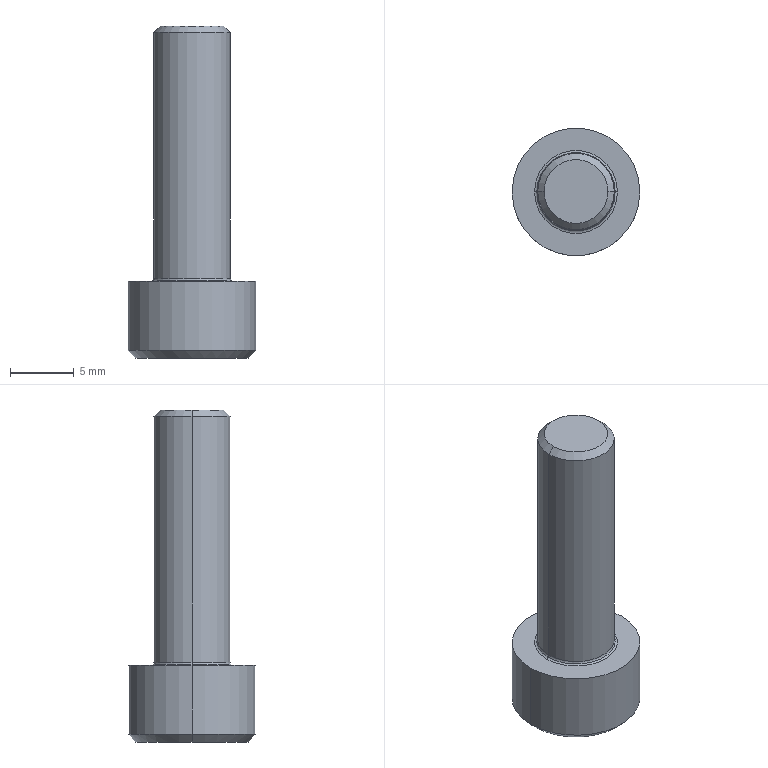Part | Creo | 1 solid | 23 faces | box 10 x 10 x 26 mm | volume 950.232 mm3 | plane 9 | cone 6 | cylinder 4 | torus 4 | commonest cylinder face diameters 6 x2 10 x2
STEP:
#1=CARTESIAN_POINT('',(-64.193,-95.403,-362.));
#2=VERTEX_POINT('',#1);
#3=CARTESIAN_POINT('',(-62.75,-92.903,-362.));
#4=VERTEX_POINT('',#3);
#5=CARTESIAN_POINT('',(-64.193,-95.403,-362.));
#6=CARTESIAN_POINT('',(-64.154,-95.335,-361.977));
#7=CARTESIAN_POINT('',(-64.077,-95.202,-361.936));
#8=CARTESIAN_POINT('',(-63.967,-95.01,-361.884));
#9=CARTESIAN_POINT('',(-63.858,-94.822,-361.842));
#10=CARTESIAN_POINT('',(-63.749,-94.633,-361.81));
#11=CARTESIAN_POINT('',(-63.639,-94.442,-361.788));
#12=CARTESIAN_POINT('',(-63.528,-94.25,-361.776));
#13=CARTESIAN_POINT('',(-63.416,-94.056,-361.776));
#14=CARTESIAN_POINT('',(-63.304,-93.863,-361.788));
#15=CARTESIAN_POINT('',(-63.194,-93.672,-361.81));
#16=CARTESIAN_POINT('',(-63.085,-93.484,-361.842));
#17=CARTESIAN_POINT('',(-62.977,-93.295,-361.884));
#18=CARTESIAN_POINT('',(-62.866,-93.103,-361.936));
#19=CARTESIAN_POINT('',(-62.789,-92.97,-361.977));
#20=CARTESIAN_POINT('',(-62.75,-92.903,-362.));
#21=B_SPLINE_CURVE_WITH_KNOTS('',3,(#5,#6,#7,#8,#9,#10,#11,#12,#13,#14,#15,#16,#17,#18,#19,#20),.UNSPECIFIED.,.F.,.F.,(4,1,1,1,1,1,1,1,1,1,1,1,1,4),(0.,0.07692,0.1538,0.2308,0.3077,0.3846,0.4615,0.5385,0.6154,0.6923,0.7692,0.8462,0.9231,1.),.UNSPECIFIED.);
#22=EDGE_CURVE('',#2,#4,#21,.T.);
#23=ORIENTED_EDGE('',*,*,#22,.F.);
#24=CARTESIAN_POINT('',(-61.307,-95.403,-360.333));
#25=VERTEX_POINT('',#24);
#26=CARTESIAN_POINT('',(-61.307,-95.403,-360.333));
#27=DIRECTION('',(-0.866,0.,-0.5));
#28=VECTOR('',#27,3.333);
#29=LINE('',#26,#28);
#30=EDGE_CURVE('',#25,#2,#29,.T.);
#31=ORIENTED_EDGE('',*,*,#30,.F.);
#32=CARTESIAN_POINT('',(-58.42,-95.403,-362.));
#33=VERTEX_POINT('',#32);
#34=CARTESIAN_POINT('',(-61.307,-95.403,-360.333));
#35=DIRECTION('',(0.866,0.,-0.5));
#36=VECTOR('',#35,3.333);
#37=LINE('',#34,#36);
#38=EDGE_CURVE('',#25,#33,#37,.T.);
#39=ORIENTED_EDGE('',*,*,#38,.T.);
#40=CARTESIAN_POINT('',(-59.863,-92.903,-362.));
#41=VERTEX_POINT('',#40);
#42=CARTESIAN_POINT('',(-59.863,-92.903,-362.));
#43=CARTESIAN_POINT('',(-59.824,-92.97,-361.977));
#44=CARTESIAN_POINT('',(-59.747,-93.103,-361.936));
#45=CARTESIAN_POINT('',(-59.637,-93.295,-361.884));
#46=CARTESIAN_POINT('',(-59.528,-93.484,-361.842));
#47=CARTESIAN_POINT('',(-59.419,-93.672,-361.81));
#48=CARTESIAN_POINT('',(-59.309,-93.863,-361.788));
#49=CARTESIAN_POINT('',(-59.197,-94.056,-361.776));
#50=CARTESIAN_POINT('',(-59.086,-94.25,-361.776));
#51=CARTESIAN_POINT('',(-58.974,-94.442,-361.788));
#52=CARTESIAN_POINT('',(-58.864,-94.633,-361.81));
#53=CARTESIAN_POINT('',(-58.755,-94.822,-361.842));
#54=CARTESIAN_POINT('',(-58.646,-95.01,-361.884));
#55=CARTESIAN_POINT('',(-58.536,-95.202,-361.936));
#56=CARTESIAN_POINT('',(-58.459,-95.335,-361.977));
#57=CARTESIAN_POINT('',(-58.42,-95.403,-362.));
#58=B_SPLINE_CURVE_WITH_KNOTS('',3,(#42,#43,#44,#45,#46,#47,#48,#49,#50,#51,#52,#53,#54,#55,#56,#57),.UNSPECIFIED.,.F.,.F.,(4,1,1,1,1,1,1,1,1,1,1,1,1,4),(0.,0.07692,0.1538,0.2308,0.3077,0.3846,0.4615,0.5385,0.6154,0.6923,0.7692,0.8462,0.9231,1.),.UNSPECIFIED.);
#59=EDGE_CURVE('',#41,#33,#58,.T.);
#60=ORIENTED_EDGE('',*,*,#59,.F.);
#61=CARTESIAN_POINT('',(-62.75,-92.903,-362.));
#62=CARTESIAN_POINT('',(-62.672,-92.903,-361.978));
#63=CARTESIAN_POINT('',(-62.519,-92.903,-361.936));
#64=CARTESIAN_POINT('',(-62.297,-92.903,-361.884));
#65=CARTESIAN_POINT('',(-62.08,-92.903,-361.843));
#66=CARTESIAN_POINT('',(-61.862,-92.903,-361.81));
#67=CARTESIAN_POINT('',(-61.642,-92.903,-361.788));
#68=CARTESIAN_POINT('',(-61.419,-92.903,-361.776));
#69=CARTESIAN_POINT('',(-61.194,-92.903,-361.776));
#70=CARTESIAN_POINT('',(-60.972,-92.903,-361.788));
#71=CARTESIAN_POINT('',(-60.751,-92.903,-361.81));
#72=CARTESIAN_POINT('',(-60.533,-92.903,-361.843));
#73=CARTESIAN_POINT('',(-60.316,-92.903,-361.884));
#74=CARTESIAN_POINT('',(-60.094,-92.903,-361.936));
#75=CARTESIAN_POINT('',(-59.941,-92.903,-361.978));
#76=CARTESIAN_POINT('',(-59.863,-92.903,-362.));
#77=B_SPLINE_CURVE_WITH_KNOTS('',3,(#61,#62,#63,#64,#65,#66,#67,#68,#69,#70,#71,#72,#73,#74,#75,#76),.UNSPECIFIED.,.F.,.F.,(4,1,1,1,1,1,1,1,1,1,1,1,1,4),(0.,0.07692,0.1538,0.2308,0.3077,0.3846,0.4615,0.5385,0.6154,0.6923,0.7692,0.8462,0.9231,1.),.UNSPECIFIED.);
#78=EDGE_CURVE('',#4,#41,#77,.T.);
#79=ORIENTED_EDGE('',*,*,#78,.F.);
#80=EDGE_LOOP('',(#23,#31,#39,#60,#79));
#81=FACE_OUTER_BOUND('',#80,.F.);
#82=CARTESIAN_POINT('',(-61.307,-95.403,-361.183));
#83=DIRECTION('',(0.,0.,-1.));
#84=DIRECTION('',(-1.,0.,0.));
#85=AXIS2_PLACEMENT_3D('',#82,#83,#84);
#86=CONICAL_SURFACE('',#85,1.472,60.);
#87=ADVANCED_FACE('',(#81),#86,.F.);
#88=CARTESIAN_POINT('',(-62.75,-92.903,-365.));
#89=VERTEX_POINT('',#88);
#90=CARTESIAN_POINT('',(-64.193,-95.403,-365.));
#91=VERTEX_POINT('',#90);
#92=CARTESIAN_POINT('',(-62.75,-92.903,-365.));
#93=DIRECTION('',(-0.5,-0.866,0.));
#94=VECTOR('',#93,2.887);
#95=LINE('',#92,#94);
#96=EDGE_CURVE('',#89,#91,#95,.T.);
#97=ORIENTED_EDGE('',*,*,#96,.T.);
#98=CARTESIAN_POINT('',(-64.193,-95.403,-365.));
#99=DIRECTION('',(0.,0.,1.));
#100=VECTOR('',#99,3.);
#101=LINE('',#98,#100);
#102=EDGE_CURVE('',#91,#2,#101,.T.);
#103=ORIENTED_EDGE('',*,*,#102,.T.);
#104=ORIENTED_EDGE('',*,*,#22,.T.);
#105=CARTESIAN_POINT('',(-62.75,-92.903,-365.));
#106=DIRECTION('',(0.,0.,1.));
#107=VECTOR('',#106,3.);
#108=LINE('',#105,#107);
#109=EDGE_CURVE('',#89,#4,#108,.T.);
#110=ORIENTED_EDGE('',*,*,#109,.F.);
#111=EDGE_LOOP('',(#97,#103,#104,#110));
#112=FACE_OUTER_BOUND('',#111,.F.);
#113=CARTESIAN_POINT('',(-62.75,-92.903,-362.));
#114=DIRECTION('',(0.866,-0.5,0.));
#115=DIRECTION('',(-0.5,-0.866,0.));
#116=AXIS2_PLACEMENT_3D('',#113,#114,#115);
#117=PLANE('',#116);
#118=ADVANCED_FACE('',(#112),#117,.T.);
#119=CARTESIAN_POINT('',(-65.707,-95.403,-365.));
#120=VERTEX_POINT('',#119);
#121=CARTESIAN_POINT('',(-56.907,-95.403,-365.));
#122=VERTEX_POINT('',#121);
#123=CARTESIAN_POINT('',(-61.307,-95.403,-365.));
#124=DIRECTION('',(0.,0.,-1.));
#125=DIRECTION('',(-1.,0.,0.));
#126=AXIS2_PLACEMENT_3D('',#123,#124,#125);
#127=CIRCLE('',#126,4.4);
#128=EDGE_CURVE('',#120,#122,#127,.T.);
#129=ORIENTED_EDGE('',*,*,#128,.F.);
#130=CARTESIAN_POINT('',(-61.307,-95.403,-365.));
#131=DIRECTION('',(0.,0.,-1.));
#132=DIRECTION('',(1.,0.,0.));
#133=AXIS2_PLACEMENT_3D('',#130,#131,#132);
#134=CIRCLE('',#133,4.4);
#135=EDGE_CURVE('',#122,#120,#134,.T.);
#136=ORIENTED_EDGE('',*,*,#135,.F.);
#137=EDGE_LOOP('',(#129,#136));
#138=FACE_OUTER_BOUND('',#137,.F.);
#139=CARTESIAN_POINT('',(-62.75,-97.903,-365.));
#140=VERTEX_POINT('',#139);
#141=CARTESIAN_POINT('',(-64.193,-95.403,-365.));
#142=DIRECTION('',(0.5,-0.866,0.));
#143=VECTOR('',#142,2.887);
#144=LINE('',#141,#143);
#145=EDGE_CURVE('',#91,#140,#144,.T.);
#146=ORIENTED_EDGE('',*,*,#145,.F.);
#147=ORIENTED_EDGE('',*,*,#96,.F.);
#148=CARTESIAN_POINT('',(-59.863,-92.903,-365.));
#149=VERTEX_POINT('',#148);
#150=CARTESIAN_POINT('',(-62.75,-92.903,-365.));
#151=DIRECTION('',(1.,0.,0.));
#152=VECTOR('',#151,2.887);
#153=LINE('',#150,#152);
#154=EDGE_CURVE('',#89,#149,#153,.T.);
#155=ORIENTED_EDGE('',*,*,#154,.T.);
#156=CARTESIAN_POINT('',(-58.42,-95.403,-365.));
#157=VERTEX_POINT('',#156);
#158=CARTESIAN_POINT('',(-58.42,-95.403,-365.));
#159=DIRECTION('',(-0.5,0.866,0.));
#160=VECTOR('',#159,2.887);
#161=LINE('',#158,#160);
#162=EDGE_CURVE('',#157,#149,#161,.T.);
#163=ORIENTED_EDGE('',*,*,#162,.F.);
#164=CARTESIAN_POINT('',(-59.863,-97.903,-365.));
#165=VERTEX_POINT('',#164);
#166=CARTESIAN_POINT('',(-59.863,-97.903,-365.));
#167=DIRECTION('',(0.5,0.866,0.));
#168=VECTOR('',#167,2.887);
#169=LINE('',#166,#168);
#170=EDGE_CURVE('',#165,#157,#169,.T.);
#171=ORIENTED_EDGE('',*,*,#170,.F.);
#172=CARTESIAN_POINT('',(-59.863,-97.903,-365.));
#173=DIRECTION('',(-1.,0.,0.));
#174=VECTOR('',#173,2.887);
#175=LINE('',#172,#174);
#176=EDGE_CURVE('',#165,#140,#175,.T.);
#177=ORIENTED_EDGE('',*,*,#176,.T.);
#178=EDGE_LOOP('',(#146,#147,#155,#163,#171,#177));
#179=FACE_BOUND('',#178,.F.);
#180=CARTESIAN_POINT('',(-61.307,-95.403,-365.));
#181=DIRECTION('',(0.,0.,-1.));
#182=DIRECTION('',(-1.,0.,0.));
#183=AXIS2_PLACEMENT_3D('',#180,#181,#182);
#184=PLANE('',#183);
#185=ADVANCED_FACE('',(#138,#179),#184,.T.);
#186=CARTESIAN_POINT('',(-66.307,-95.403,-364.4));
#187=VERTEX_POINT('',#186);
#188=CARTESIAN_POINT('',(-56.307,-95.403,-364.4));
#189=VERTEX_POINT('',#188);
#190=CARTESIAN_POINT('',(-61.307,-95.403,-364.4));
#191=DIRECTION('',(0.,0.,-1.));
#192=DIRECTION('',(-1.,0.,0.));
#193=AXIS2_PLACEMENT_3D('',#190,#191,#192);
#194=CIRCLE('',#193,5.);
#195=EDGE_CURVE('',#187,#189,#194,.T.);
#196=ORIENTED_EDGE('',*,*,#195,.F.);
#197=CARTESIAN_POINT('',(-65.707,-95.403,-365.));
#198=DIRECTION('',(-0.7071,0.,0.7071));
#199=VECTOR('',#198,0.8485);
#200=LINE('',#197,#199);
#201=EDGE_CURVE('',#120,#187,#200,.T.);
#202=ORIENTED_EDGE('',*,*,#201,.F.);
#203=ORIENTED_EDGE('',*,*,#128,.T.);
#204=CARTESIAN_POINT('',(-56.907,-95.403,-365.));
#205=DIRECTION('',(0.7071,0.,0.7071));
#206=VECTOR('',#205,0.8485);
#207=LINE('',#204,#206);
#208=EDGE_CURVE('',#122,#189,#207,.T.);
#209=ORIENTED_EDGE('',*,*,#208,.T.);
#210=EDGE_LOOP('',(#196,#202,#203,#209));
#211=FACE_OUTER_BOUND('',#210,.F.);
#212=CARTESIAN_POINT('',(-61.307,-95.403,-364.7));
#213=DIRECTION('',(0.,0.,1.));
#214=DIRECTION('',(1.,0.,0.));
#215=AXIS2_PLACEMENT_3D('',#212,#213,#214);
#216=CONICAL_SURFACE('',#215,4.7,45.);
#217=ADVANCED_FACE('',(#211),#216,.T.);
#218=ORIENTED_EDGE('',*,*,#195,.T.);
#219=CARTESIAN_POINT('',(-56.307,-95.403,-359.));
#220=VERTEX_POINT('',#219);
#221=CARTESIAN_POINT('',(-56.307,-95.403,-359.));
#222=DIRECTION('',(0.,0.,-1.));
#223=VECTOR('',#222,5.4);
#224=LINE('',#221,#223);
#225=EDGE_CURVE('',#220,#189,#224,.T.);
#226=ORIENTED_EDGE('',*,*,#225,.F.);
#227=CARTESIAN_POINT('',(-66.307,-95.403,-359.));
#228=VERTEX_POINT('',#227);
#229=CARTESIAN_POINT('',(-61.307,-95.403,-359.));
#230=DIRECTION('',(0.,0.,1.));
#231=DIRECTION('',(1.,0.,0.));
#232=AXIS2_PLACEMENT_3D('',#229,#230,#231);
#233=CIRCLE('',#232,5.);
#234=EDGE_CURVE('',#220,#228,#233,.T.);
#235=ORIENTED_EDGE('',*,*,#234,.T.);
#236=CARTESIAN_POINT('',(-66.307,-95.403,-359.));
#237=DIRECTION('',(0.,0.,-1.));
#238=VECTOR('',#237,5.4);
#239=LINE('',#236,#238);
#240=EDGE_CURVE('',#228,#187,#239,.T.);
#241=ORIENTED_EDGE('',*,*,#240,.T.);
#242=EDGE_LOOP('',(#218,#226,#235,#241));
#243=FACE_OUTER_BOUND('',#242,.F.);
#244=CARTESIAN_POINT('',(-61.307,-95.403,-359.));
#245=DIRECTION('',(0.,0.,-1.));
#246=DIRECTION('',(-1.,0.,0.));
#247=AXIS2_PLACEMENT_3D('',#244,#245,#246);
#248=CYLINDRICAL_SURFACE('',#247,5.);
#249=ADVANCED_FACE('',(#243),#248,.T.);
#250=CARTESIAN_POINT('',(-61.307,-95.403,-364.4));
#251=DIRECTION('',(0.,0.,-1.));
#252=DIRECTION('',(1.,0.,0.));
#253=AXIS2_PLACEMENT_3D('',#250,#251,#252);
#254=CIRCLE('',#253,5.);
#255=EDGE_CURVE('',#189,#187,#254,.T.);
#256=ORIENTED_EDGE('',*,*,#255,.T.);
#257=ORIENTED_EDGE('',*,*,#240,.F.);
#258=CARTESIAN_POINT('',(-61.307,-95.403,-359.));
#259=DIRECTION('',(0.,0.,1.));
#260=DIRECTION('',(-1.,0.,0.));
#261=AXIS2_PLACEMENT_3D('',#258,#259,#260);
#262=CIRCLE('',#261,5.);
#263=EDGE_CURVE('',#228,#220,#262,.T.);
#264=ORIENTED_EDGE('',*,*,#263,.T.);
#265=ORIENTED_EDGE('',*,*,#225,.T.);
#266=EDGE_LOOP('',(#256,#257,#264,#265));
#267=FACE_OUTER_BOUND('',#266,.F.);
#268=CARTESIAN_POINT('',(-61.307,-95.403,-359.));
#269=DIRECTION('',(0.,0.,-1.));
#270=DIRECTION('',(-1.,0.,0.));
#271=AXIS2_PLACEMENT_3D('',#268,#269,#270);
#272=CYLINDRICAL_SURFACE('',#271,5.);
#273=ADVANCED_FACE('',(#267),#272,.T.);
#274=ORIENTED_EDGE('',*,*,#255,.F.);
#275=ORIENTED_EDGE('',*,*,#208,.F.);
#276=ORIENTED_EDGE('',*,*,#135,.T.);
#277=ORIENTED_EDGE('',*,*,#201,.T.);
#278=EDGE_LOOP('',(#274,#275,#276,#277));
#279=FACE_OUTER_BOUND('',#278,.F.);
#280=CARTESIAN_POINT('',(-61.307,-95.403,-364.7));
#281=DIRECTION('',(0.,0.,1.));
#282=DIRECTION('',(1.,0.,0.));
#283=AXIS2_PLACEMENT_3D('',#280,#281,#282);
#284=CONICAL_SURFACE('',#283,4.7,45.);
#285=ADVANCED_FACE('',(#279),#284,.T.);
#286=ORIENTED_EDGE('',*,*,#263,.F.);
#287=ORIENTED_EDGE('',*,*,#234,.F.);
#288=EDGE_LOOP('',(#286,#287));
#289=FACE_OUTER_BOUND('',#288,.F.);
#290=CARTESIAN_POINT('',(-64.557,-95.403,-359.));
#291=VERTEX_POINT('',#290);
#292=CARTESIAN_POINT('',(-58.057,-95.403,-359.));
#293=VERTEX_POINT('',#292);
#294=CARTESIAN_POINT('',(-61.307,-95.403,-359.));
#295=DIRECTION('',(0.,0.,-1.));
#296=DIRECTION('',(-1.,0.,0.));
#297=AXIS2_PLACEMENT_3D('',#294,#295,#296);
#298=CIRCLE('',#297,3.25);
#299=EDGE_CURVE('',#291,#293,#298,.T.);
#300=ORIENTED_EDGE('',*,*,#299,.F.);
#301=CARTESIAN_POINT('',(-61.307,-95.403,-359.));
#302=DIRECTION('',(0.,0.,-1.));
#303=DIRECTION('',(1.,0.,0.));
#304=AXIS2_PLACEMENT_3D('',#301,#302,#303);
#305=CIRCLE('',#304,3.25);
#306=EDGE_CURVE('',#293,#291,#305,.T.);
#307=ORIENTED_EDGE('',*,*,#306,.F.);
#308=EDGE_LOOP('',(#300,#307));
#309=FACE_BOUND('',#308,.F.);
#310=CARTESIAN_POINT('',(-61.307,-95.403,-359.));
#311=DIRECTION('',(0.,0.,-1.));
#312=DIRECTION('',(-1.,0.,0.));
#313=AXIS2_PLACEMENT_3D('',#310,#311,#312);
#314=PLANE('',#313);
#315=ADVANCED_FACE('',(#289,#309),#314,.F.);
#316=ORIENTED_EDGE('',*,*,#299,.T.);
#317=CARTESIAN_POINT('',(-58.233,-95.403,-358.927));
#318=VERTEX_POINT('',#317);
#319=CARTESIAN_POINT('',(-58.057,-95.403,-358.75));
#320=DIRECTION('',(0.,1.,0.));
#321=DIRECTION('',(0.,0.,-1.));
#322=AXIS2_PLACEMENT_3D('',#319,#320,#321);
#323=CIRCLE('',#322,0.25);
#324=EDGE_CURVE('',#293,#318,#323,.T.);
#325=ORIENTED_EDGE('',*,*,#324,.T.);
#326=CARTESIAN_POINT('',(-64.38,-95.403,-358.927));
#327=VERTEX_POINT('',#326);
#328=CARTESIAN_POINT('',(-61.307,-95.403,-358.927));
#329=DIRECTION('',(0.,0.,-1.));
#330=DIRECTION('',(-1.,0.,0.));
#331=AXIS2_PLACEMENT_3D('',#328,#329,#330);
#332=CIRCLE('',#331,3.073);
#333=EDGE_CURVE('',#327,#318,#332,.T.);
#334=ORIENTED_EDGE('',*,*,#333,.F.);
#335=CARTESIAN_POINT('',(-64.557,-95.403,-358.75));
#336=DIRECTION('',(0.,-1.,0.));
#337=DIRECTION('',(0.,0.,-1.));
#338=AXIS2_PLACEMENT_3D('',#335,#336,#337);
#339=CIRCLE('',#338,0.25);
#340=EDGE_CURVE('',#291,#327,#339,.T.);
#341=ORIENTED_EDGE('',*,*,#340,.F.);
#342=EDGE_LOOP('',(#316,#325,#334,#341));
#343=FACE_OUTER_BOUND('',#342,.F.);
#344=CARTESIAN_POINT('',(-61.307,-95.403,-358.75));
#345=DIRECTION('',(0.,0.,-1.));
#346=DIRECTION('',(-1.,0.,0.));
#347=AXIS2_PLACEMENT_3D('',#344,#345,#346);
#348=TOROIDAL_SURFACE('',#347,3.25,0.25);
#349=ADVANCED_FACE('',(#343),#348,.F.);
#350=ORIENTED_EDGE('',*,*,#306,.T.);
#351=ORIENTED_EDGE('',*,*,#340,.T.);
#352=CARTESIAN_POINT('',(-61.307,-95.403,-358.927));
#353=DIRECTION('',(0.,0.,-1.));
#354=DIRECTION('',(1.,0.,0.));
#355=AXIS2_PLACEMENT_3D('',#352,#353,#354);
#356=CIRCLE('',#355,3.073);
#357=EDGE_CURVE('',#318,#327,#356,.T.);
#358=ORIENTED_EDGE('',*,*,#357,.F.);
#359=ORIENTED_EDGE('',*,*,#324,.F.);
#360=EDGE_LOOP('',(#350,#351,#358,#359));
#361=FACE_OUTER_BOUND('',#360,.F.);
#362=CARTESIAN_POINT('',(-61.307,-95.403,-358.75));
#363=DIRECTION('',(0.,0.,-1.));
#364=DIRECTION('',(-1.,0.,0.));
#365=AXIS2_PLACEMENT_3D('',#362,#363,#364);
#366=TOROIDAL_SURFACE('',#365,3.25,0.25);
#367=ADVANCED_FACE('',(#361),#366,.F.);
#368=CARTESIAN_POINT('',(-58.307,-95.403,-358.75));
#369=VERTEX_POINT('',#368);
#370=CARTESIAN_POINT('',(-64.307,-95.403,-358.75));
#371=VERTEX_POINT('',#370);
#372=CARTESIAN_POINT('',(-61.307,-95.403,-358.75));
#373=DIRECTION('',(0.,0.,-1.));
#374=DIRECTION('',(1.,0.,0.));
#375=AXIS2_PLACEMENT_3D('',#372,#373,#374);
#376=CIRCLE('',#375,3.);
#377=EDGE_CURVE('',#369,#371,#376,.T.);
#378=ORIENTED_EDGE('',*,*,#377,.F.);
#379=CARTESIAN_POINT('',(-58.057,-95.403,-358.75));
#380=DIRECTION('',(0.,1.,0.));
#381=DIRECTION('',(-0.7071,0.,-0.7071));
#382=AXIS2_PLACEMENT_3D('',#379,#380,#381);
#383=CIRCLE('',#382,0.25);
#384=EDGE_CURVE('',#318,#369,#383,.T.);
#385=ORIENTED_EDGE('',*,*,#384,.F.);
#386=ORIENTED_EDGE('',*,*,#357,.T.);
#387=CARTESIAN_POINT('',(-64.557,-95.403,-358.75));
#388=DIRECTION('',(0.,-1.,0.));
#389=DIRECTION('',(0.7071,0.,-0.7071));
#390=AXIS2_PLACEMENT_3D('',#387,#388,#389);
#391=CIRCLE('',#390,0.25);
#392=EDGE_CURVE('',#327,#371,#391,.T.);
#393=ORIENTED_EDGE('',*,*,#392,.T.);
#394=EDGE_LOOP('',(#378,#385,#386,#393));
#395=FACE_OUTER_BOUND('',#394,.F.);
#396=CARTESIAN_POINT('',(-61.307,-95.403,-358.75));
#397=DIRECTION('',(0.,0.,-1.));
#398=DIRECTION('',(-1.,0.,0.));
#399=AXIS2_PLACEMENT_3D('',#396,#397,#398);
#400=TOROIDAL_SURFACE('',#399,3.25,0.25);
#401=ADVANCED_FACE('',(#395),#400,.F.);
#402=CARTESIAN_POINT('',(-64.307,-95.403,-339.5));
#403=VERTEX_POINT('',#402);
#404=CARTESIAN_POINT('',(-58.307,-95.403,-339.5));
#405=VERTEX_POINT('',#404);
#406=CARTESIAN_POINT('',(-61.307,-95.403,-339.5));
#407=DIRECTION('',(0.,0.,1.));
#408=DIRECTION('',(-1.,0.,0.));
#409=AXIS2_PLACEMENT_3D('',#406,#407,#408);
#410=CIRCLE('',#409,3.);
#411=EDGE_CURVE('',#403,#405,#410,.T.);
#412=ORIENTED_EDGE('',*,*,#411,.T.);
#413=CARTESIAN_POINT('',(-58.307,-95.403,-339.5));
#414=DIRECTION('',(0.,0.,-1.));
#415=VECTOR('',#414,19.25);
#416=LINE('',#413,#415);
#417=EDGE_CURVE('',#405,#369,#416,.T.);
#418=ORIENTED_EDGE('',*,*,#417,.T.);
#419=ORIENTED_EDGE('',*,*,#377,.T.);
#420=CARTESIAN_POINT('',(-64.307,-95.403,-339.5));
#421=DIRECTION('',(0.,0.,-1.));
#422=VECTOR('',#421,19.25);
#423=LINE('',#420,#422);
#424=EDGE_CURVE('',#403,#371,#423,.T.);
#425=ORIENTED_EDGE('',*,*,#424,.F.);
#426=EDGE_LOOP('',(#412,#418,#419,#425));
#427=FACE_OUTER_BOUND('',#426,.F.);
#428=CARTESIAN_POINT('',(-61.307,-95.403,-339.));
#429=DIRECTION('',(0.,0.,-1.));
#430=DIRECTION('',(-1.,0.,0.));
#431=AXIS2_PLACEMENT_3D('',#428,#429,#430);
#432=CYLINDRICAL_SURFACE('',#431,3.);
#433=ADVANCED_FACE('',(#427),#432,.T.);
#434=CARTESIAN_POINT('',(-63.807,-95.403,-339.));
#435=VERTEX_POINT('',#434);
#436=CARTESIAN_POINT('',(-58.807,-95.403,-339.));
#437=VERTEX_POINT('',#436);
#438=CARTESIAN_POINT('',(-61.307,-95.403,-339.));
#439=DIRECTION('',(0.,0.,1.));
#440=DIRECTION('',(-1.,0.,0.));
#441=AXIS2_PLACEMENT_3D('',#438,#439,#440);
#442=CIRCLE('',#441,2.5);
#443=EDGE_CURVE('',#435,#437,#442,.T.);
#444=ORIENTED_EDGE('',*,*,#443,.T.);
#445=CARTESIAN_POINT('',(-58.807,-95.403,-339.));
#446=DIRECTION('',(0.7071,0.,-0.7071));
#447=VECTOR('',#446,0.7071);
#448=LINE('',#445,#447);
#449=EDGE_CURVE('',#437,#405,#448,.T.);
#450=ORIENTED_EDGE('',*,*,#449,.T.);
#451=ORIENTED_EDGE('',*,*,#411,.F.);
#452=CARTESIAN_POINT('',(-63.807,-95.403,-339.));
#453=DIRECTION('',(-0.7071,0.,-0.7071));
#454=VECTOR('',#453,0.7071);
#455=LINE('',#452,#454);
#456=EDGE_CURVE('',#435,#403,#455,.T.);
#457=ORIENTED_EDGE('',*,*,#456,.F.);
#458=EDGE_LOOP('',(#444,#450,#451,#457));
#459=FACE_OUTER_BOUND('',#458,.F.);
#460=CARTESIAN_POINT('',(-61.307,-95.403,-339.25));
#461=DIRECTION('',(0.,0.,-1.));
#462=DIRECTION('',(-1.,0.,0.));
#463=AXIS2_PLACEMENT_3D('',#460,#461,#462);
#464=CONICAL_SURFACE('',#463,2.75,45.);
#465=ADVANCED_FACE('',(#459),#464,.T.);
#466=ORIENTED_EDGE('',*,*,#443,.F.);
#467=CARTESIAN_POINT('',(-61.307,-95.403,-339.));
#468=DIRECTION('',(0.,0.,1.));
#469=DIRECTION('',(1.,0.,0.));
#470=AXIS2_PLACEMENT_3D('',#467,#468,#469);
#471=CIRCLE('',#470,2.5);
#472=EDGE_CURVE('',#437,#435,#471,.T.);
#473=ORIENTED_EDGE('',*,*,#472,.F.);
#474=EDGE_LOOP('',(#466,#473));
#475=FACE_OUTER_BOUND('',#474,.F.);
#476=CARTESIAN_POINT('',(-61.307,-95.403,-339.));
#477=DIRECTION('',(0.,0.,-1.));
#478=DIRECTION('',(-1.,0.,0.));
#479=AXIS2_PLACEMENT_3D('',#476,#477,#478);
#480=PLANE('',#479);
#481=ADVANCED_FACE('',(#475),#480,.F.);
#482=ORIENTED_EDGE('',*,*,#472,.T.);
#483=ORIENTED_EDGE('',*,*,#456,.T.);
#484=CARTESIAN_POINT('',(-61.307,-95.403,-339.5));
#485=DIRECTION('',(0.,0.,1.));
#486=DIRECTION('',(1.,0.,0.));
#487=AXIS2_PLACEMENT_3D('',#484,#485,#486);
#488=CIRCLE('',#487,3.);
#489=EDGE_CURVE('',#405,#403,#488,.T.);
#490=ORIENTED_EDGE('',*,*,#489,.F.);
#491=ORIENTED_EDGE('',*,*,#449,.F.);
#492=EDGE_LOOP('',(#482,#483,#490,#491));
#493=FACE_OUTER_BOUND('',#492,.F.);
#494=CARTESIAN_POINT('',(-61.307,-95.403,-339.25));
#495=DIRECTION('',(0.,0.,-1.));
#496=DIRECTION('',(-1.,0.,0.));
#497=AXIS2_PLACEMENT_3D('',#494,#495,#496);
#498=CONICAL_SURFACE('',#497,2.75,45.);
#499=ADVANCED_FACE('',(#493),#498,.T.);
#500=ORIENTED_EDGE('',*,*,#489,.T.);
#501=ORIENTED_EDGE('',*,*,#424,.T.);
#502=CARTESIAN_POINT('',(-61.307,-95.403,-358.75));
#503=DIRECTION('',(0.,0.,-1.));
#504=DIRECTION('',(-1.,0.,0.));
#505=AXIS2_PLACEMENT_3D('',#502,#503,#504);
#506=CIRCLE('',#505,3.);
#507=EDGE_CURVE('',#371,#369,#506,.T.);
#508=ORIENTED_EDGE('',*,*,#507,.T.);
#509=ORIENTED_EDGE('',*,*,#417,.F.);
#510=EDGE_LOOP('',(#500,#501,#508,#509));
#511=FACE_OUTER_BOUND('',#510,.F.);
#512=CARTESIAN_POINT('',(-61.307,-95.403,-339.));
#513=DIRECTION('',(0.,0.,-1.));
#514=DIRECTION('',(-1.,0.,0.));
#515=AXIS2_PLACEMENT_3D('',#512,#513,#514);
#516=CYLINDRICAL_SURFACE('',#515,3.);
#517=ADVANCED_FACE('',(#511),#516,.T.);
#518=ORIENTED_EDGE('',*,*,#507,.F.);
#519=ORIENTED_EDGE('',*,*,#392,.F.);
#520=ORIENTED_EDGE('',*,*,#333,.T.);
#521=ORIENTED_EDGE('',*,*,#384,.T.);
#522=EDGE_LOOP('',(#518,#519,#520,#521));
#523=FACE_OUTER_BOUND('',#522,.F.);
#524=CARTESIAN_POINT('',(-61.307,-95.403,-358.75));
#525=DIRECTION('',(0.,0.,-1.));
#526=DIRECTION('',(-1.,0.,0.));
#527=AXIS2_PLACEMENT_3D('',#524,#525,#526);
#528=TOROIDAL_SURFACE('',#527,3.25,0.25);
#529=ADVANCED_FACE('',(#523),#528,.F.);
#530=ORIENTED_EDGE('',*,*,#145,.T.);
#531=CARTESIAN_POINT('',(-62.75,-97.903,-362.));
#532=VERTEX_POINT('',#531);
#533=CARTESIAN_POINT('',(-62.75,-97.903,-365.));
#534=DIRECTION('',(0.,0.,1.));
#535=VECTOR('',#534,3.);
#536=LINE('',#533,#535);
#537=EDGE_CURVE('',#140,#532,#536,.T.);
#538=ORIENTED_EDGE('',*,*,#537,.T.);
#539=CARTESIAN_POINT('',(-62.75,-97.903,-362.));
#540=CARTESIAN_POINT('',(-62.789,-97.835,-361.977));
#541=CARTESIAN_POINT('',(-62.866,-97.702,-361.936));
#542=CARTESIAN_POINT('',(-62.977,-97.51,-361.884));
#543=CARTESIAN_POINT('',(-63.085,-97.322,-361.842));
#544=CARTESIAN_POINT('',(-63.194,-97.133,-361.81));
#545=CARTESIAN_POINT('',(-63.304,-96.942,-361.788));
#546=CARTESIAN_POINT('',(-63.416,-96.75,-361.776));
#547=CARTESIAN_POINT('',(-63.528,-96.556,-361.776));
#548=CARTESIAN_POINT('',(-63.639,-96.363,-361.788));
#549=CARTESIAN_POINT('',(-63.749,-96.172,-361.81));
#550=CARTESIAN_POINT('',(-63.858,-95.984,-361.842));
#551=CARTESIAN_POINT('',(-63.967,-95.795,-361.884));
#552=CARTESIAN_POINT('',(-64.077,-95.603,-361.936));
#553=CARTESIAN_POINT('',(-64.154,-95.47,-361.977));
#554=CARTESIAN_POINT('',(-64.193,-95.403,-362.));
#555=B_SPLINE_CURVE_WITH_KNOTS('',3,(#539,#540,#541,#542,#543,#544,#545,#546,#547,#548,#549,#550,#551,#552,#553,#554),.UNSPECIFIED.,.F.,.F.,(4,1,1,1,1,1,1,1,1,1,1,1,1,4),(0.,0.07692,0.1538,0.2308,0.3077,0.3846,0.4615,0.5385,0.6154,0.6923,0.7692,0.8462,0.9231,1.),.UNSPECIFIED.);
#556=EDGE_CURVE('',#532,#2,#555,.T.);
#557=ORIENTED_EDGE('',*,*,#556,.T.);
#558=ORIENTED_EDGE('',*,*,#102,.F.);
#559=EDGE_LOOP('',(#530,#538,#557,#558));
#560=FACE_OUTER_BOUND('',#559,.F.);
#561=CARTESIAN_POINT('',(-64.193,-95.403,-362.));
#562=DIRECTION('',(0.866,0.5,0.));
#563=DIRECTION('',(0.5,-0.866,0.));
#564=AXIS2_PLACEMENT_3D('',#561,#562,#563);
#565=PLANE('',#564);
#566=ADVANCED_FACE('',(#560),#565,.T.);
#567=ORIENTED_EDGE('',*,*,#176,.F.);
#568=CARTESIAN_POINT('',(-59.863,-97.903,-362.));
#569=VERTEX_POINT('',#568);
#570=CARTESIAN_POINT('',(-59.863,-97.903,-365.));
#571=DIRECTION('',(0.,0.,1.));
#572=VECTOR('',#571,3.);
#573=LINE('',#570,#572);
#574=EDGE_CURVE('',#165,#569,#573,.T.);
#575=ORIENTED_EDGE('',*,*,#574,.T.);
#576=CARTESIAN_POINT('',(-59.863,-97.903,-362.));
#577=CARTESIAN_POINT('',(-59.941,-97.903,-361.978));
#578=CARTESIAN_POINT('',(-60.094,-97.903,-361.936));
#579=CARTESIAN_POINT('',(-60.316,-97.903,-361.884));
#580=CARTESIAN_POINT('',(-60.533,-97.903,-361.843));
#581=CARTESIAN_POINT('',(-60.751,-97.903,-361.81));
#582=CARTESIAN_POINT('',(-60.972,-97.903,-361.788));
#583=CARTESIAN_POINT('',(-61.194,-97.903,-361.776));
#584=CARTESIAN_POINT('',(-61.419,-97.903,-361.776));
#585=CARTESIAN_POINT('',(-61.642,-97.903,-361.788));
#586=CARTESIAN_POINT('',(-61.862,-97.903,-361.81));
#587=CARTESIAN_POINT('',(-62.08,-97.903,-361.843));
#588=CARTESIAN_POINT('',(-62.297,-97.903,-361.884));
#589=CARTESIAN_POINT('',(-62.519,-97.903,-361.936));
#590=CARTESIAN_POINT('',(-62.672,-97.903,-361.978));
#591=CARTESIAN_POINT('',(-62.75,-97.903,-362.));
#592=B_SPLINE_CURVE_WITH_KNOTS('',3,(#576,#577,#578,#579,#580,#581,#582,#583,#584,#585,#586,#587,#588,#589,#590,#591),.UNSPECIFIED.,.F.,.F.,(4,1,1,1,1,1,1,1,1,1,1,1,1,4),(0.,0.07692,0.1538,0.2308,0.3077,0.3846,0.4615,0.5385,0.6154,0.6923,0.7692,0.8462,0.9231,1.),.UNSPECIFIED.);
#593=EDGE_CURVE('',#569,#532,#592,.T.);
#594=ORIENTED_EDGE('',*,*,#593,.T.);
#595=ORIENTED_EDGE('',*,*,#537,.F.);
#596=EDGE_LOOP('',(#567,#575,#594,#595));
#597=FACE_OUTER_BOUND('',#596,.F.);
#598=CARTESIAN_POINT('',(-62.75,-97.903,-362.));
#599=DIRECTION('',(0.,1.,0.));
#600=DIRECTION('',(0.,0.,-1.));
#601=AXIS2_PLACEMENT_3D('',#598,#599,#600);
#602=PLANE('',#601);
#603=ADVANCED_FACE('',(#597),#602,.T.);
#604=ORIENTED_EDGE('',*,*,#170,.T.);
#605=CARTESIAN_POINT('',(-58.42,-95.403,-365.));
#606=DIRECTION('',(0.,0.,1.));
#607=VECTOR('',#606,3.);
#608=LINE('',#605,#607);
#609=EDGE_CURVE('',#157,#33,#608,.T.);
#610=ORIENTED_EDGE('',*,*,#609,.T.);
#611=CARTESIAN_POINT('',(-58.42,-95.403,-362.));
#612=CARTESIAN_POINT('',(-58.459,-95.47,-361.977));
#613=CARTESIAN_POINT('',(-58.536,-95.603,-361.936));
#614=CARTESIAN_POINT('',(-58.646,-95.795,-361.884));
#615=CARTESIAN_POINT('',(-58.755,-95.984,-361.842));
#616=CARTESIAN_POINT('',(-58.864,-96.172,-361.81));
#617=CARTESIAN_POINT('',(-58.974,-96.363,-361.788));
#618=CARTESIAN_POINT('',(-59.086,-96.556,-361.776));
#619=CARTESIAN_POINT('',(-59.197,-96.75,-361.776));
#620=CARTESIAN_POINT('',(-59.309,-96.942,-361.788));
#621=CARTESIAN_POINT('',(-59.419,-97.133,-361.81));
#622=CARTESIAN_POINT('',(-59.528,-97.322,-361.842));
#623=CARTESIAN_POINT('',(-59.637,-97.51,-361.884));
#624=CARTESIAN_POINT('',(-59.747,-97.702,-361.936));
#625=CARTESIAN_POINT('',(-59.824,-97.835,-361.977));
#626=CARTESIAN_POINT('',(-59.863,-97.903,-362.));
#627=B_SPLINE_CURVE_WITH_KNOTS('',3,(#611,#612,#613,#614,#615,#616,#617,#618,#619,#620,#621,#622,#623,#624,#625,#626),.UNSPECIFIED.,.F.,.F.,(4,1,1,1,1,1,1,1,1,1,1,1,1,4),(0.,0.07692,0.1538,0.2308,0.3077,0.3846,0.4615,0.5385,0.6154,0.6923,0.7692,0.8462,0.9231,1.),.UNSPECIFIED.);
#628=EDGE_CURVE('',#33,#569,#627,.T.);
#629=ORIENTED_EDGE('',*,*,#628,.T.);
#630=ORIENTED_EDGE('',*,*,#574,.F.);
#631=EDGE_LOOP('',(#604,#610,#629,#630));
#632=FACE_OUTER_BOUND('',#631,.F.);
#633=CARTESIAN_POINT('',(-59.863,-97.903,-362.));
#634=DIRECTION('',(-0.866,0.5,0.));
#635=DIRECTION('',(0.5,0.866,0.));
#636=AXIS2_PLACEMENT_3D('',#633,#634,#635);
#637=PLANE('',#636);
#638=ADVANCED_FACE('',(#632),#637,.T.);
#639=ORIENTED_EDGE('',*,*,#162,.T.);
#640=CARTESIAN_POINT('',(-59.863,-92.903,-365.));
#641=DIRECTION('',(0.,0.,1.));
#642=VECTOR('',#641,3.);
#643=LINE('',#640,#642);
#644=EDGE_CURVE('',#149,#41,#643,.T.);
#645=ORIENTED_EDGE('',*,*,#644,.T.);
#646=ORIENTED_EDGE('',*,*,#59,.T.);
#647=ORIENTED_EDGE('',*,*,#609,.F.);
#648=EDGE_LOOP('',(#639,#645,#646,#647));
#649=FACE_OUTER_BOUND('',#648,.F.);
#650=CARTESIAN_POINT('',(-58.42,-95.403,-362.));
#651=DIRECTION('',(-0.866,-0.5,0.));
#652=DIRECTION('',(-0.5,0.866,0.));
#653=AXIS2_PLACEMENT_3D('',#650,#651,#652);
#654=PLANE('',#653);
#655=ADVANCED_FACE('',(#649),#654,.T.);
#656=ORIENTED_EDGE('',*,*,#154,.F.);
#657=ORIENTED_EDGE('',*,*,#109,.T.);
#658=ORIENTED_EDGE('',*,*,#78,.T.);
#659=ORIENTED_EDGE('',*,*,#644,.F.);
#660=EDGE_LOOP('',(#656,#657,#658,#659));
#661=FACE_OUTER_BOUND('',#660,.F.);
#662=CARTESIAN_POINT('',(-59.863,-92.903,-362.));
#663=DIRECTION('',(0.,-1.,0.));
#664=DIRECTION('',(0.,0.,1.));
#665=AXIS2_PLACEMENT_3D('',#662,#663,#664);
#666=PLANE('',#665);
#667=ADVANCED_FACE('',(#661),#666,.T.);
#668=ORIENTED_EDGE('',*,*,#628,.F.);
#669=ORIENTED_EDGE('',*,*,#38,.F.);
#670=ORIENTED_EDGE('',*,*,#30,.T.);
#671=ORIENTED_EDGE('',*,*,#556,.F.);
#672=ORIENTED_EDGE('',*,*,#593,.F.);
#673=EDGE_LOOP('',(#668,#669,#670,#671,#672));
#674=FACE_OUTER_BOUND('',#673,.F.);
#675=CARTESIAN_POINT('',(-61.307,-95.403,-361.183));
#676=DIRECTION('',(0.,0.,-1.));
#677=DIRECTION('',(-1.,0.,0.));
#678=AXIS2_PLACEMENT_3D('',#675,#676,#677);
#679=CONICAL_SURFACE('',#678,1.472,60.);
#680=ADVANCED_FACE('',(#674),#679,.F.);
#681=CLOSED_SHELL('',(#87,#118,#185,#217,#249,#273,#285,#315,#349,#367,#401,#433,#465,#481,#499,#517,#529,#566,#603,#638,#655,#667,#680));
#682=MANIFOLD_SOLID_BREP('',#681);
#683=(LENGTH_UNIT()NAMED_UNIT(*)SI_UNIT(.MILLI.,.METRE.));
#684=UNCERTAINTY_MEASURE_WITH_UNIT(LENGTH_MEASURE(0.00296),#683,'','');
#685=(NAMED_UNIT(*)PLANE_ANGLE_UNIT()SI_UNIT($,.RADIAN.));
#686=PLANE_ANGLE_MEASURE_WITH_UNIT(PLANE_ANGLE_MEASURE(0.01745),#685);
#687=(CONVERSION_BASED_UNIT('DEGREE',#686)NAMED_UNIT(*)PLANE_ANGLE_UNIT());
#688=(NAMED_UNIT(*)SI_UNIT($,.STERADIAN.)SOLID_ANGLE_UNIT());
#689=(GEOMETRIC_REPRESENTATION_CONTEXT(3)GLOBAL_UNCERTAINTY_ASSIGNED_CONTEXT((#684))GLOBAL_UNIT_ASSIGNED_CONTEXT((#683,#687,#688))REPRESENTATION_CONTEXT('',''));
#690=ADVANCED_BREP_SHAPE_REPRESENTATION('',(#682),#689);